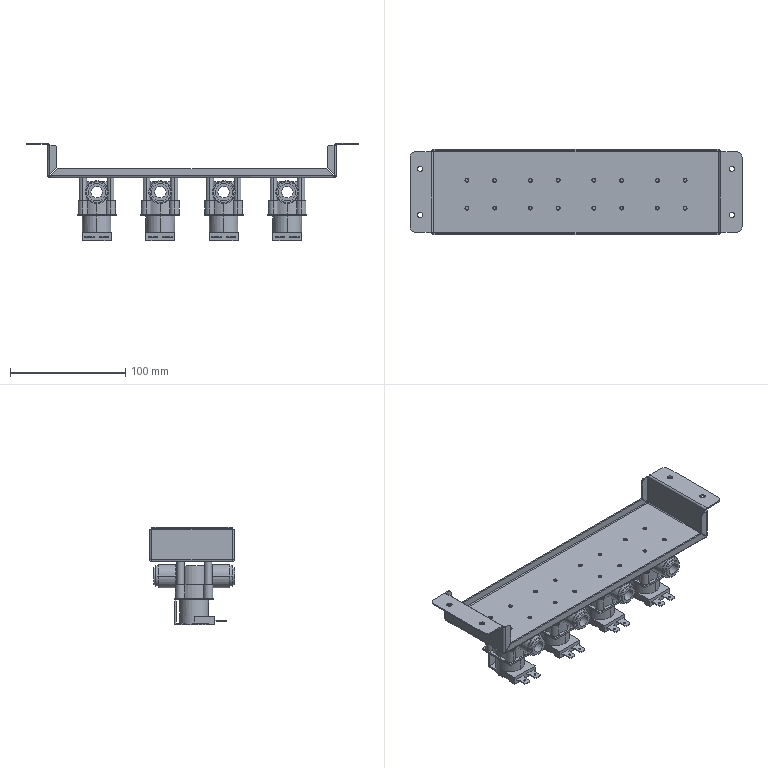Part | SolidWorks | features ReferencePattern 3, AEMSimFeature 1, LocalLPattern 1 | 5 solids | 630 faces | box 287.6 x 73.8 x 84.7 mm | volume 205450 mm3 | plane 314 | cylinder 308 | spline 8 | commonest cylinder face diameters 3.4 x34 2.8 x32 6.5 x32 8.5 x24 31.5 x20 1.7 x16